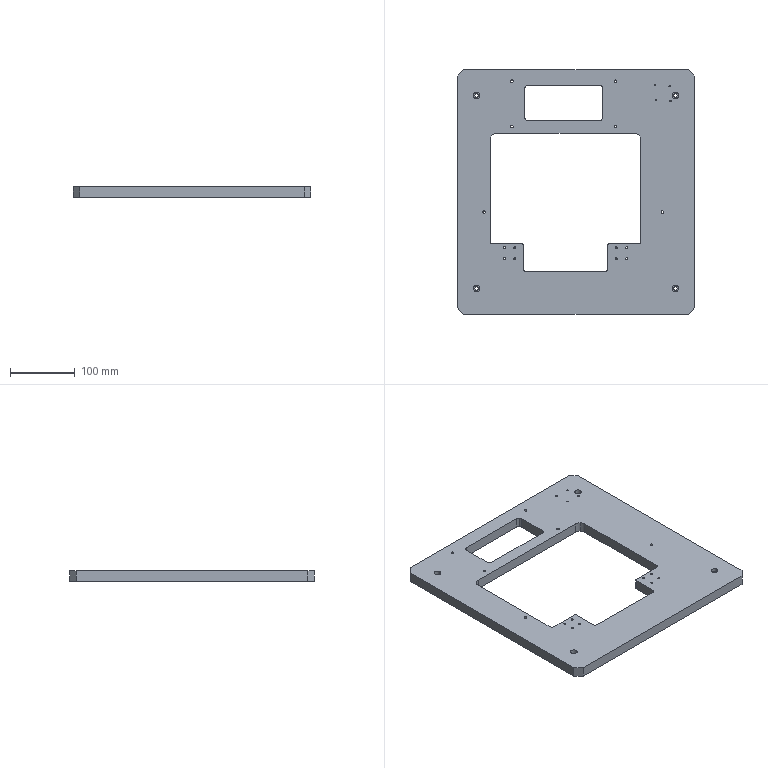Part | STEP file | ASND-0110-TCTF01-23 | 1 solid | 100 faces | box 366.812 x 377.833 x 16 mm | volume 1379157 mm3 | cylinder 74 | plane 26 | commonest cylinder face diameters 4 x20 10 x18 3 x16 2 x8 5.5 x8 20 x4